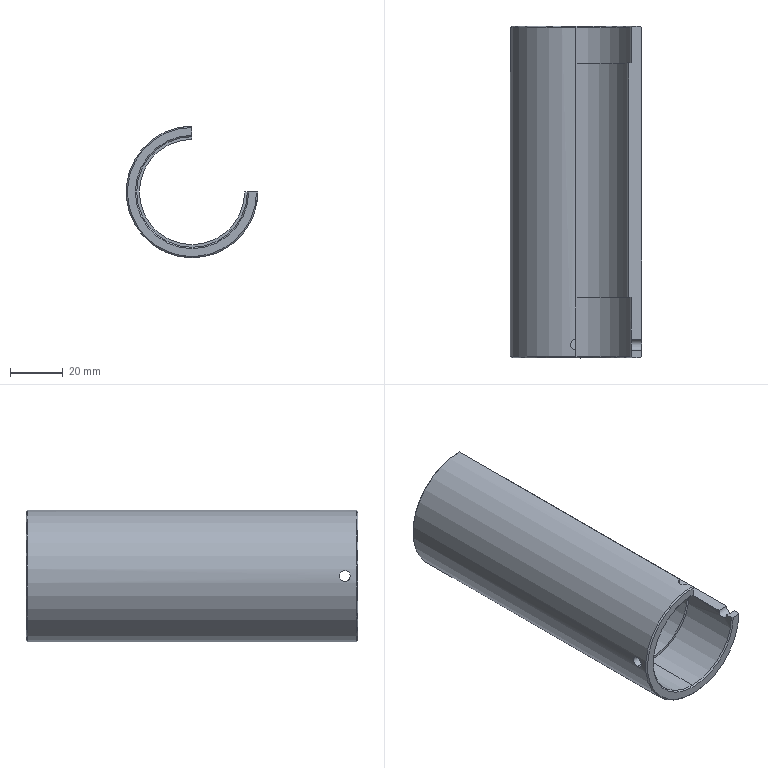Part | STEP file | 1 solid | 26 faces | box 50 x 126 x 50 mm | volume 63059 mm3 | cylinder 12 | plane 8 | cone 6 | commonest cylinder face diameters 4.2 x5 42 x3 40 x2 50 x2